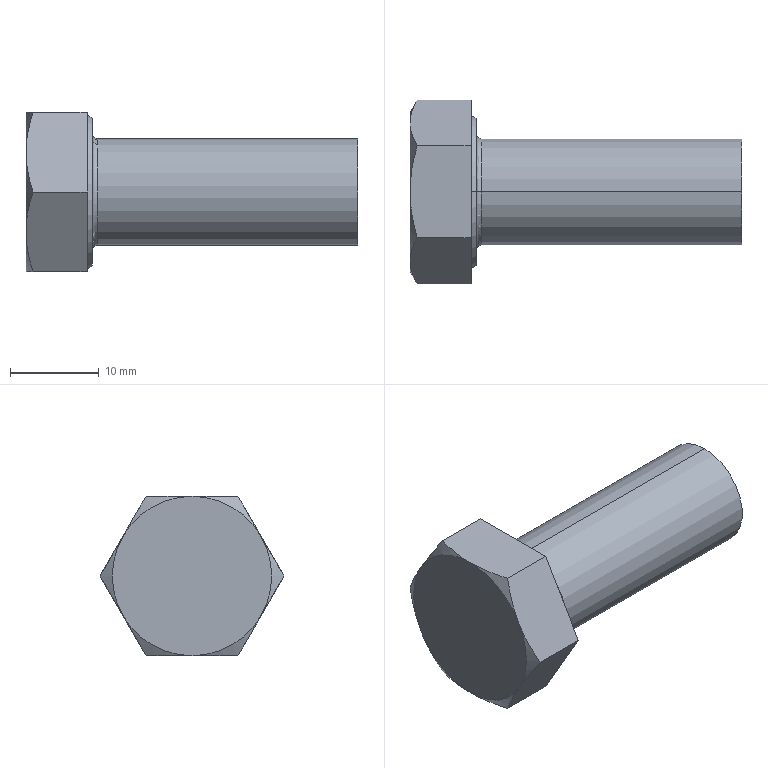Part | SolidWorks | features RevCut 3, Extrusion 1, Fillet 1, LPattern 1, Revolution 1 | 1 solid | 22 faces | box 37.5 x 20.785 x 18 mm | volume 5461 mm3 | plane 10 | cone 8 | torus 2 | cylinder 2 | commonest cylinder face diameters 12 x2
STEP:
#1=CARTESIAN_POINT('',(8.1,0.,6.));
#2=VERTEX_POINT('',#1);
#3=CARTESIAN_POINT('',(8.1,0.,-6.));
#4=VERTEX_POINT('',#3);
#5=CARTESIAN_POINT('',(8.1,0.,0.));
#6=DIRECTION('',(1.,0.,0.));
#7=DIRECTION('',(0.,0.,-1.));
#8=AXIS2_PLACEMENT_3D('',#5,#6,#7);
#9=CIRCLE('',#8,6.);
#10=EDGE_CURVE('',#2,#4,#9,.T.);
#11=ORIENTED_EDGE('',*,*,#10,.F.);
#12=CARTESIAN_POINT('',(7.5,0.,6.6));
#13=VERTEX_POINT('',#12);
#14=CARTESIAN_POINT('',(8.1,0.,6.6));
#15=DIRECTION('',(0.,1.,0.));
#16=DIRECTION('',(0.,0.,1.));
#17=AXIS2_PLACEMENT_3D('',#14,#15,#16);
#18=CIRCLE('',#17,0.6);
#19=EDGE_CURVE('',#2,#13,#18,.T.);
#20=ORIENTED_EDGE('',*,*,#19,.T.);
#21=CARTESIAN_POINT('',(7.5,0.,-6.6));
#22=VERTEX_POINT('',#21);
#23=CARTESIAN_POINT('',(7.5,0.,0.));
#24=DIRECTION('',(-1.,0.,0.));
#25=DIRECTION('',(0.,0.,-1.));
#26=AXIS2_PLACEMENT_3D('',#23,#24,#25);
#27=CIRCLE('',#26,6.6);
#28=EDGE_CURVE('',#22,#13,#27,.T.);
#29=ORIENTED_EDGE('',*,*,#28,.F.);
#30=CARTESIAN_POINT('',(8.1,0.,-6.6));
#31=DIRECTION('',(0.,-1.,0.));
#32=DIRECTION('',(0.,0.,-1.));
#33=AXIS2_PLACEMENT_3D('',#30,#31,#32);
#34=CIRCLE('',#33,0.6);
#35=EDGE_CURVE('',#4,#22,#34,.T.);
#36=ORIENTED_EDGE('',*,*,#35,.F.);
#37=EDGE_LOOP('',(#11,#20,#29,#36));
#38=FACE_OUTER_BOUND('',#37,.T.);
#39=CARTESIAN_POINT('',(8.1,0.,0.));
#40=DIRECTION('',(1.,0.,0.));
#41=DIRECTION('',(0.,0.,-1.));
#42=AXIS2_PLACEMENT_3D('',#39,#40,#41);
#43=TOROIDAL_SURFACE('',#42,6.6,0.6);
#44=ADVANCED_FACE('',(#38),#43,.F.);
#45=CARTESIAN_POINT('',(37.5,0.,6.));
#46=VERTEX_POINT('',#45);
#47=CARTESIAN_POINT('',(37.5,0.,-6.));
#48=VERTEX_POINT('',#47);
#49=CARTESIAN_POINT('',(37.5,0.,0.));
#50=DIRECTION('',(-1.,0.,0.));
#51=DIRECTION('',(0.,0.,1.));
#52=AXIS2_PLACEMENT_3D('',#49,#50,#51);
#53=CIRCLE('',#52,6.);
#54=EDGE_CURVE('',#46,#48,#53,.T.);
#55=ORIENTED_EDGE('',*,*,#54,.T.);
#56=CARTESIAN_POINT('',(0.,0.,-6.));
#57=DIRECTION('',(-1.,0.,0.));
#58=VECTOR('',#57,1000.);
#59=LINE('',#56,#58);
#60=EDGE_CURVE('',#48,#4,#59,.T.);
#61=ORIENTED_EDGE('',*,*,#60,.T.);
#62=CARTESIAN_POINT('',(8.1,0.,0.));
#63=DIRECTION('',(1.,0.,0.));
#64=DIRECTION('',(0.,0.,-1.));
#65=AXIS2_PLACEMENT_3D('',#62,#63,#64);
#66=CIRCLE('',#65,6.);
#67=EDGE_CURVE('',#4,#2,#66,.T.);
#68=ORIENTED_EDGE('',*,*,#67,.T.);
#69=CARTESIAN_POINT('',(0.,0.,6.));
#70=DIRECTION('',(-1.,0.,0.));
#71=VECTOR('',#70,1000.);
#72=LINE('',#69,#71);
#73=EDGE_CURVE('',#46,#2,#72,.T.);
#74=ORIENTED_EDGE('',*,*,#73,.F.);
#75=EDGE_LOOP('',(#55,#61,#68,#74));
#76=FACE_OUTER_BOUND('',#75,.T.);
#77=CARTESIAN_POINT('',(0.,0.,0.));
#78=DIRECTION('',(-1.,0.,0.));
#79=DIRECTION('',(0.,0.,1.));
#80=AXIS2_PLACEMENT_3D('',#77,#78,#79);
#81=CYLINDRICAL_SURFACE('',#80,6.);
#82=ADVANCED_FACE('',(#76),#81,.T.);
#83=CARTESIAN_POINT('',(7.5,0.,8.315));
#84=VERTEX_POINT('',#83);
#85=CARTESIAN_POINT('',(7.5,0.,-8.315));
#86=VERTEX_POINT('',#85);
#87=CARTESIAN_POINT('',(7.5,0.,0.));
#88=DIRECTION('',(-1.,0.,0.));
#89=DIRECTION('',(0.,0.,1.));
#90=AXIS2_PLACEMENT_3D('',#87,#88,#89);
#91=CIRCLE('',#90,8.315);
#92=EDGE_CURVE('',#84,#86,#91,.T.);
#93=ORIENTED_EDGE('',*,*,#92,.T.);
#94=CARTESIAN_POINT('',(6.9,0.,-8.661));
#95=VERTEX_POINT('',#94);
#96=CARTESIAN_POINT('',(6.9,0.,-8.661));
#97=DIRECTION('',(-0.866,0.,-0.5));
#98=VECTOR('',#97,1000.);
#99=LINE('',#96,#98);
#100=EDGE_CURVE('',#86,#95,#99,.T.);
#101=ORIENTED_EDGE('',*,*,#100,.T.);
#102=CARTESIAN_POINT('',(6.9,0.,8.661));
#103=VERTEX_POINT('',#102);
#104=CARTESIAN_POINT('',(6.9,0.,0.));
#105=DIRECTION('',(-1.,0.,0.));
#106=DIRECTION('',(0.,0.,1.));
#107=AXIS2_PLACEMENT_3D('',#104,#105,#106);
#108=CIRCLE('',#107,8.661);
#109=EDGE_CURVE('',#103,#95,#108,.T.);
#110=ORIENTED_EDGE('',*,*,#109,.F.);
#111=CARTESIAN_POINT('',(6.9,0.,8.661));
#112=DIRECTION('',(-0.866,0.,0.5));
#113=VECTOR('',#112,1000.);
#114=LINE('',#111,#113);
#115=EDGE_CURVE('',#84,#103,#114,.T.);
#116=ORIENTED_EDGE('',*,*,#115,.F.);
#117=EDGE_LOOP('',(#93,#101,#110,#116));
#118=FACE_OUTER_BOUND('',#117,.T.);
#119=CARTESIAN_POINT('',(6.9,0.,0.));
#120=DIRECTION('',(-1.,0.,0.));
#121=DIRECTION('',(0.,0.,1.));
#122=AXIS2_PLACEMENT_3D('',#119,#120,#121);
#123=CONICAL_SURFACE('',#122,8.661,0.5236);
#124=ADVANCED_FACE('',(#118),#123,.T.);
#125=CARTESIAN_POINT('',(6.9,5.196,-9.));
#126=VERTEX_POINT('',#125);
#127=CARTESIAN_POINT('',(6.9,10.392,0.));
#128=VERTEX_POINT('',#127);
#129=CARTESIAN_POINT('',(6.9,5.196,-9.));
#130=DIRECTION('',(0.,0.5,0.866));
#131=VECTOR('',#130,1000.);
#132=LINE('',#129,#131);
#133=EDGE_CURVE('',#126,#128,#132,.T.);
#134=ORIENTED_EDGE('',*,*,#133,.F.);
#135=CARTESIAN_POINT('',(0.8038,5.196,-9.));
#136=VERTEX_POINT('',#135);
#137=CARTESIAN_POINT('',(7.5,5.196,-9.));
#138=DIRECTION('',(-1.,0.,0.));
#139=VECTOR('',#138,1000.);
#140=LINE('',#137,#139);
#141=EDGE_CURVE('',#126,#136,#140,.T.);
#142=ORIENTED_EDGE('',*,*,#141,.T.);
#143=CARTESIAN_POINT('',(0.,7.794,-4.5));
#144=VERTEX_POINT('',#143);
#145=CARTESIAN_POINT('',(0.,7.794,-4.5));
#146=CARTESIAN_POINT('',(0.,7.574,-4.882));
#147=CARTESIAN_POINT('',(0.019,7.352,-5.266));
#148=CARTESIAN_POINT('',(0.09253,6.914,-6.024));
#149=CARTESIAN_POINT('',(0.147,6.697,-6.401));
#150=CARTESIAN_POINT('',(0.357,6.048,-7.525));
#151=CARTESIAN_POINT('',(0.5591,5.62,-8.266));
#152=CARTESIAN_POINT('',(0.8038,5.196,-9.));
#153=B_SPLINE_CURVE_WITH_KNOTS('',3,(#145,#146,#147,#148,#149,#150,#151,#152),.UNSPECIFIED.,.F.,.F.,(4,2,2,4),(0.005258,0.006567,0.007877,0.0105),.UNSPECIFIED.);
#154=EDGE_CURVE('',#144,#136,#153,.T.);
#155=ORIENTED_EDGE('',*,*,#154,.F.);
#156=CARTESIAN_POINT('',(0.8038,10.392,0.));
#157=VERTEX_POINT('',#156);
#158=CARTESIAN_POINT('',(0.8038,10.392,0.));
#159=CARTESIAN_POINT('',(0.5585,9.967,-0.7361));
#160=CARTESIAN_POINT('',(0.3563,9.539,-1.478));
#161=CARTESIAN_POINT('',(0.07661,8.674,-2.976));
#162=CARTESIAN_POINT('',(0.,8.237,-3.733));
#163=CARTESIAN_POINT('',(0.,7.794,-4.5));
#164=B_SPLINE_CURVE_WITH_KNOTS('',3,(#158,#159,#160,#161,#162,#163),.UNSPECIFIED.,.F.,.F.,(4,2,4),(0.000000238,0.002629,0.005258),.UNSPECIFIED.);
#165=EDGE_CURVE('',#157,#144,#164,.T.);
#166=ORIENTED_EDGE('',*,*,#165,.F.);
#167=CARTESIAN_POINT('',(7.5,10.392,0.));
#168=DIRECTION('',(-1.,0.,0.));
#169=VECTOR('',#168,1000.);
#170=LINE('',#167,#169);
#171=EDGE_CURVE('',#128,#157,#170,.T.);
#172=ORIENTED_EDGE('',*,*,#171,.F.);
#173=EDGE_LOOP('',(#134,#142,#155,#166,#172));
#174=FACE_OUTER_BOUND('',#173,.T.);
#175=CARTESIAN_POINT('',(7.5,5.196,-9.));
#176=DIRECTION('',(0.,-0.866,0.5));
#177=DIRECTION('',(0.,-0.5,-0.866));
#178=AXIS2_PLACEMENT_3D('',#175,#176,#177);
#179=PLANE('',#178);
#180=ADVANCED_FACE('',(#174),#179,.F.);
#181=CARTESIAN_POINT('',(6.9,5.196,9.));
#182=VERTEX_POINT('',#181);
#183=CARTESIAN_POINT('',(6.9,10.392,0.));
#184=DIRECTION('',(0.,-0.5,0.866));
#185=VECTOR('',#184,1000.);
#186=LINE('',#183,#185);
#187=EDGE_CURVE('',#128,#182,#186,.T.);
#188=ORIENTED_EDGE('',*,*,#187,.F.);
#189=ORIENTED_EDGE('',*,*,#171,.T.);
#190=CARTESIAN_POINT('',(0.,7.794,4.5));
#191=VERTEX_POINT('',#190);
#192=CARTESIAN_POINT('',(0.,7.794,4.5));
#193=CARTESIAN_POINT('',(0.,8.015,4.118));
#194=CARTESIAN_POINT('',(0.019,8.236,3.734));
#195=CARTESIAN_POINT('',(0.09253,8.674,2.976));
#196=CARTESIAN_POINT('',(0.147,8.892,2.599));
#197=CARTESIAN_POINT('',(0.357,9.541,1.475));
#198=CARTESIAN_POINT('',(0.5591,9.968,0.7343));
#199=CARTESIAN_POINT('',(0.8038,10.392,0.));
#200=B_SPLINE_CURVE_WITH_KNOTS('',3,(#192,#193,#194,#195,#196,#197,#198,#199),.UNSPECIFIED.,.F.,.F.,(4,2,2,4),(0.005258,0.006567,0.007877,0.0105),.UNSPECIFIED.);
#201=EDGE_CURVE('',#191,#157,#200,.T.);
#202=ORIENTED_EDGE('',*,*,#201,.F.);
#203=CARTESIAN_POINT('',(0.8038,5.196,9.));
#204=VERTEX_POINT('',#203);
#205=CARTESIAN_POINT('',(0.8038,5.196,9.));
#206=CARTESIAN_POINT('',(0.5585,5.621,8.264));
#207=CARTESIAN_POINT('',(0.3563,6.049,7.522));
#208=CARTESIAN_POINT('',(0.07661,6.914,6.024));
#209=CARTESIAN_POINT('',(0.,7.352,5.267));
#210=CARTESIAN_POINT('',(0.,7.794,4.5));
#211=B_SPLINE_CURVE_WITH_KNOTS('',3,(#205,#206,#207,#208,#209,#210),.UNSPECIFIED.,.F.,.F.,(4,2,4),(0.000000238,0.002629,0.005258),.UNSPECIFIED.);
#212=EDGE_CURVE('',#204,#191,#211,.T.);
#213=ORIENTED_EDGE('',*,*,#212,.F.);
#214=CARTESIAN_POINT('',(7.5,5.196,9.));
#215=DIRECTION('',(-1.,0.,0.));
#216=VECTOR('',#215,1000.);
#217=LINE('',#214,#216);
#218=EDGE_CURVE('',#182,#204,#217,.T.);
#219=ORIENTED_EDGE('',*,*,#218,.F.);
#220=EDGE_LOOP('',(#188,#189,#202,#213,#219));
#221=FACE_OUTER_BOUND('',#220,.T.);
#222=CARTESIAN_POINT('',(7.5,10.392,0.));
#223=DIRECTION('',(0.,-0.866,-0.5));
#224=DIRECTION('',(0.,0.5,-0.866));
#225=AXIS2_PLACEMENT_3D('',#222,#223,#224);
#226=PLANE('',#225);
#227=ADVANCED_FACE('',(#221),#226,.F.);
#228=CARTESIAN_POINT('',(6.9,-5.196,9.));
#229=VERTEX_POINT('',#228);
#230=CARTESIAN_POINT('',(6.9,5.196,9.));
#231=DIRECTION('',(0.,-1.,0.));
#232=VECTOR('',#231,1000.);
#233=LINE('',#230,#232);
#234=EDGE_CURVE('',#182,#229,#233,.T.);
#235=ORIENTED_EDGE('',*,*,#234,.F.);
#236=ORIENTED_EDGE('',*,*,#218,.T.);
#237=CARTESIAN_POINT('',(0.,0.,9.));
#238=VERTEX_POINT('',#237);
#239=CARTESIAN_POINT('',(0.,0.,9.));
#240=CARTESIAN_POINT('',(0.,0.4401,9.));
#241=CARTESIAN_POINT('',(0.01885,0.8832,9.));
#242=CARTESIAN_POINT('',(0.09319,1.767,9.));
#243=CARTESIAN_POINT('',(0.1482,2.204,9.));
#244=CARTESIAN_POINT('',(0.3593,3.505,9.));
#245=CARTESIAN_POINT('',(0.5612,4.356,9.));
#246=CARTESIAN_POINT('',(0.8038,5.196,9.));
#247=B_SPLINE_CURVE_WITH_KNOTS('',3,(#239,#240,#241,#242,#243,#244,#245,#246),.UNSPECIFIED.,.F.,.F.,(4,2,2,4),(0.01498,0.0163,0.01761,0.02025),.UNSPECIFIED.);
#248=EDGE_CURVE('',#238,#204,#247,.T.);
#249=ORIENTED_EDGE('',*,*,#248,.F.);
#250=CARTESIAN_POINT('',(0.8038,-5.196,9.));
#251=VERTEX_POINT('',#250);
#252=CARTESIAN_POINT('',(0.8038,-5.196,9.));
#253=CARTESIAN_POINT('',(0.5595,-4.35,9.));
#254=CARTESIAN_POINT('',(0.3552,-3.485,9.));
#255=CARTESIAN_POINT('',(0.07569,-1.752,9.));
#256=CARTESIAN_POINT('',(0.,-0.8794,9.));
#257=CARTESIAN_POINT('',(0.,0.,9.));
#258=B_SPLINE_CURVE_WITH_KNOTS('',3,(#252,#253,#254,#255,#256,#257),.UNSPECIFIED.,.F.,.F.,(4,2,4),(0.00972,0.01235,0.01498),.UNSPECIFIED.);
#259=EDGE_CURVE('',#251,#238,#258,.T.);
#260=ORIENTED_EDGE('',*,*,#259,.F.);
#261=CARTESIAN_POINT('',(7.5,-5.196,9.));
#262=DIRECTION('',(-1.,0.,0.));
#263=VECTOR('',#262,1000.);
#264=LINE('',#261,#263);
#265=EDGE_CURVE('',#229,#251,#264,.T.);
#266=ORIENTED_EDGE('',*,*,#265,.F.);
#267=EDGE_LOOP('',(#235,#236,#249,#260,#266));
#268=FACE_OUTER_BOUND('',#267,.T.);
#269=CARTESIAN_POINT('',(7.5,5.196,9.));
#270=DIRECTION('',(0.,0.,-1.));
#271=DIRECTION('',(-1.,0.,0.));
#272=AXIS2_PLACEMENT_3D('',#269,#270,#271);
#273=PLANE('',#272);
#274=ADVANCED_FACE('',(#268),#273,.F.);
#275=CARTESIAN_POINT('',(6.9,-10.392,0.));
#276=VERTEX_POINT('',#275);
#277=CARTESIAN_POINT('',(6.9,-10.392,0.));
#278=DIRECTION('',(0.,-0.5,-0.866));
#279=VECTOR('',#278,1000.);
#280=LINE('',#277,#279);
#281=EDGE_CURVE('',#229,#276,#280,.T.);
#282=ORIENTED_EDGE('',*,*,#281,.F.);
#283=ORIENTED_EDGE('',*,*,#265,.T.);
#284=CARTESIAN_POINT('',(0.,-7.794,4.5));
#285=VERTEX_POINT('',#284);
#286=CARTESIAN_POINT('',(0.,-7.794,4.5));
#287=CARTESIAN_POINT('',(0.,-7.574,4.882));
#288=CARTESIAN_POINT('',(0.019,-7.352,5.266));
#289=CARTESIAN_POINT('',(0.09253,-6.914,6.024));
#290=CARTESIAN_POINT('',(0.147,-6.697,6.401));
#291=CARTESIAN_POINT('',(0.357,-6.048,7.525));
#292=CARTESIAN_POINT('',(0.5591,-5.62,8.266));
#293=CARTESIAN_POINT('',(0.8038,-5.196,9.));
#294=B_SPLINE_CURVE_WITH_KNOTS('',3,(#286,#287,#288,#289,#290,#291,#292,#293),.UNSPECIFIED.,.F.,.F.,(4,2,2,4),(0.005258,0.006567,0.007877,0.0105),.UNSPECIFIED.);
#295=EDGE_CURVE('',#285,#251,#294,.T.);
#296=ORIENTED_EDGE('',*,*,#295,.F.);
#297=CARTESIAN_POINT('',(0.8038,-10.392,0.));
#298=VERTEX_POINT('',#297);
#299=CARTESIAN_POINT('',(0.8038,-10.392,0.));
#300=CARTESIAN_POINT('',(0.5585,-9.967,0.7361));
#301=CARTESIAN_POINT('',(0.3563,-9.539,1.478));
#302=CARTESIAN_POINT('',(0.07661,-8.674,2.976));
#303=CARTESIAN_POINT('',(0.,-8.237,3.733));
#304=CARTESIAN_POINT('',(0.,-7.794,4.5));
#305=B_SPLINE_CURVE_WITH_KNOTS('',3,(#299,#300,#301,#302,#303,#304),.UNSPECIFIED.,.F.,.F.,(4,2,4),(0.000000238,0.002629,0.005258),.UNSPECIFIED.);
#306=EDGE_CURVE('',#298,#285,#305,.T.);
#307=ORIENTED_EDGE('',*,*,#306,.F.);
#308=CARTESIAN_POINT('',(7.5,-10.392,0.));
#309=DIRECTION('',(-1.,0.,0.));
#310=VECTOR('',#309,1000.);
#311=LINE('',#308,#310);
#312=EDGE_CURVE('',#276,#298,#311,.T.);
#313=ORIENTED_EDGE('',*,*,#312,.F.);
#314=EDGE_LOOP('',(#282,#283,#296,#307,#313));
#315=FACE_OUTER_BOUND('',#314,.T.);
#316=CARTESIAN_POINT('',(7.5,-10.392,0.));
#317=DIRECTION('',(0.,0.866,-0.5));
#318=DIRECTION('',(0.,0.5,0.866));
#319=AXIS2_PLACEMENT_3D('',#316,#317,#318);
#320=PLANE('',#319);
#321=ADVANCED_FACE('',(#315),#320,.F.);
#322=CARTESIAN_POINT('',(6.9,-5.196,-9.));
#323=VERTEX_POINT('',#322);
#324=CARTESIAN_POINT('',(6.9,-5.196,-9.));
#325=DIRECTION('',(0.,0.5,-0.866));
#326=VECTOR('',#325,1000.);
#327=LINE('',#324,#326);
#328=EDGE_CURVE('',#276,#323,#327,.T.);
#329=ORIENTED_EDGE('',*,*,#328,.F.);
#330=ORIENTED_EDGE('',*,*,#312,.T.);
#331=CARTESIAN_POINT('',(0.,-7.794,-4.5));
#332=VERTEX_POINT('',#331);
#333=CARTESIAN_POINT('',(0.,-7.794,-4.5));
#334=CARTESIAN_POINT('',(0.,-8.015,-4.118));
#335=CARTESIAN_POINT('',(0.019,-8.236,-3.734));
#336=CARTESIAN_POINT('',(0.09253,-8.674,-2.976));
#337=CARTESIAN_POINT('',(0.147,-8.892,-2.599));
#338=CARTESIAN_POINT('',(0.357,-9.541,-1.475));
#339=CARTESIAN_POINT('',(0.5591,-9.968,-0.7343));
#340=CARTESIAN_POINT('',(0.8038,-10.392,0.));
#341=B_SPLINE_CURVE_WITH_KNOTS('',3,(#333,#334,#335,#336,#337,#338,#339,#340),.UNSPECIFIED.,.F.,.F.,(4,2,2,4),(0.005258,0.006567,0.007877,0.0105),.UNSPECIFIED.);
#342=EDGE_CURVE('',#332,#298,#341,.T.);
#343=ORIENTED_EDGE('',*,*,#342,.F.);
#344=CARTESIAN_POINT('',(0.8038,-5.196,-9.));
#345=VERTEX_POINT('',#344);
#346=CARTESIAN_POINT('',(0.8038,-5.196,-9.));
#347=CARTESIAN_POINT('',(0.5585,-5.621,-8.264));
#348=CARTESIAN_POINT('',(0.3563,-6.049,-7.522));
#349=CARTESIAN_POINT('',(0.07661,-6.914,-6.024));
#350=CARTESIAN_POINT('',(0.,-7.352,-5.267));
#351=CARTESIAN_POINT('',(0.,-7.794,-4.5));
#352=B_SPLINE_CURVE_WITH_KNOTS('',3,(#346,#347,#348,#349,#350,#351),.UNSPECIFIED.,.F.,.F.,(4,2,4),(0.000000238,0.002629,0.005258),.UNSPECIFIED.);
#353=EDGE_CURVE('',#345,#332,#352,.T.);
#354=ORIENTED_EDGE('',*,*,#353,.F.);
#355=CARTESIAN_POINT('',(7.5,-5.196,-9.));
#356=DIRECTION('',(-1.,0.,0.));
#357=VECTOR('',#356,1000.);
#358=LINE('',#355,#357);
#359=EDGE_CURVE('',#323,#345,#358,.T.);
#360=ORIENTED_EDGE('',*,*,#359,.F.);
#361=EDGE_LOOP('',(#329,#330,#343,#354,#360));
#362=FACE_OUTER_BOUND('',#361,.T.);
#363=CARTESIAN_POINT('',(7.5,-5.196,-9.));
#364=DIRECTION('',(0.,0.866,0.5));
#365=DIRECTION('',(0.,-0.5,0.866));
#366=AXIS2_PLACEMENT_3D('',#363,#364,#365);
#367=PLANE('',#366);
#368=ADVANCED_FACE('',(#362),#367,.F.);
#369=CARTESIAN_POINT('',(6.9,5.196,-9.));
#370=DIRECTION('',(0.,1.,0.));
#371=VECTOR('',#370,1000.);
#372=LINE('',#369,#371);
#373=EDGE_CURVE('',#323,#126,#372,.T.);
#374=ORIENTED_EDGE('',*,*,#373,.F.);
#375=ORIENTED_EDGE('',*,*,#359,.T.);
#376=CARTESIAN_POINT('',(0.,0.,-9.));
#377=VERTEX_POINT('',#376);
#378=CARTESIAN_POINT('',(0.,0.,-9.));
#379=CARTESIAN_POINT('',(0.,-0.8794,-9.));
#380=CARTESIAN_POINT('',(0.07569,-1.752,-9.));
#381=CARTESIAN_POINT('',(0.3552,-3.485,-9.));
#382=CARTESIAN_POINT('',(0.5595,-4.35,-9.));
#383=CARTESIAN_POINT('',(0.8038,-5.196,-9.));
#384=B_SPLINE_CURVE_WITH_KNOTS('',3,(#378,#379,#380,#381,#382,#383),.UNSPECIFIED.,.F.,.F.,(4,2,4),(0.03045,0.03308,0.03571),.UNSPECIFIED.);
#385=EDGE_CURVE('',#377,#345,#384,.T.);
#386=ORIENTED_EDGE('',*,*,#385,.F.);
#387=CARTESIAN_POINT('',(0.8038,5.196,-9.));
#388=CARTESIAN_POINT('',(0.5612,4.356,-9.));
#389=CARTESIAN_POINT('',(0.3593,3.505,-9.));
#390=CARTESIAN_POINT('',(0.1482,2.204,-9.));
#391=CARTESIAN_POINT('',(0.09319,1.767,-9.));
#392=CARTESIAN_POINT('',(0.01885,0.8832,-9.));
#393=CARTESIAN_POINT('',(0.,0.4401,-9.));
#394=CARTESIAN_POINT('',(0.,0.,-9.));
#395=B_SPLINE_CURVE_WITH_KNOTS('',3,(#387,#388,#389,#390,#391,#392,#393,#394),.UNSPECIFIED.,.F.,.F.,(4,2,2,4),(0.02519,0.02782,0.02914,0.03045),.UNSPECIFIED.);
#396=EDGE_CURVE('',#136,#377,#395,.T.);
#397=ORIENTED_EDGE('',*,*,#396,.F.);
#398=ORIENTED_EDGE('',*,*,#141,.F.);
#399=EDGE_LOOP('',(#374,#375,#386,#397,#398));
#400=FACE_OUTER_BOUND('',#399,.T.);
#401=CARTESIAN_POINT('',(7.5,5.196,-9.));
#402=DIRECTION('',(0.,0.,1.));
#403=DIRECTION('',(0.,-1.,0.));
#404=AXIS2_PLACEMENT_3D('',#401,#402,#403);
#405=PLANE('',#404);
#406=ADVANCED_FACE('',(#400),#405,.F.);
#407=ORIENTED_EDGE('',*,*,#353,.T.);
#408=CARTESIAN_POINT('',(0.,0.,0.));
#409=DIRECTION('',(1.,0.,0.));
#410=DIRECTION('',(0.,0.,-1.));
#411=AXIS2_PLACEMENT_3D('',#408,#409,#410);
#412=CIRCLE('',#411,9.);
#413=EDGE_CURVE('',#332,#377,#412,.T.);
#414=ORIENTED_EDGE('',*,*,#413,.T.);
#415=ORIENTED_EDGE('',*,*,#385,.T.);
#416=EDGE_LOOP('',(#407,#414,#415));
#417=FACE_OUTER_BOUND('',#416,.T.);
#418=CARTESIAN_POINT('',(0.,0.,0.));
#419=DIRECTION('',(1.,0.,0.));
#420=DIRECTION('',(0.,0.,-1.));
#421=AXIS2_PLACEMENT_3D('',#418,#419,#420);
#422=CONICAL_SURFACE('',#421,9.,1.047);
#423=ADVANCED_FACE('',(#417),#422,.T.);
#424=ORIENTED_EDGE('',*,*,#306,.T.);
#425=CARTESIAN_POINT('',(0.,0.,0.));
#426=DIRECTION('',(1.,0.,0.));
#427=DIRECTION('',(0.,0.,-1.));
#428=AXIS2_PLACEMENT_3D('',#425,#426,#427);
#429=CIRCLE('',#428,9.);
#430=EDGE_CURVE('',#285,#332,#429,.T.);
#431=ORIENTED_EDGE('',*,*,#430,.T.);
#432=ORIENTED_EDGE('',*,*,#342,.T.);
#433=EDGE_LOOP('',(#424,#431,#432));
#434=FACE_OUTER_BOUND('',#433,.T.);
#435=CARTESIAN_POINT('',(0.,0.,0.));
#436=DIRECTION('',(1.,0.,0.));
#437=DIRECTION('',(0.,0.,-1.));
#438=AXIS2_PLACEMENT_3D('',#435,#436,#437);
#439=CONICAL_SURFACE('',#438,9.,1.047);
#440=ADVANCED_FACE('',(#434),#439,.T.);
#441=ORIENTED_EDGE('',*,*,#259,.T.);
#442=CARTESIAN_POINT('',(0.,0.,0.));
#443=DIRECTION('',(1.,0.,0.));
#444=DIRECTION('',(0.,0.,-1.));
#445=AXIS2_PLACEMENT_3D('',#442,#443,#444);
#446=CIRCLE('',#445,9.);
#447=EDGE_CURVE('',#238,#285,#446,.T.);
#448=ORIENTED_EDGE('',*,*,#447,.T.);
#449=ORIENTED_EDGE('',*,*,#295,.T.);
#450=EDGE_LOOP('',(#441,#448,#449));
#451=FACE_OUTER_BOUND('',#450,.T.);
#452=CARTESIAN_POINT('',(0.,0.,0.));
#453=DIRECTION('',(1.,0.,0.));
#454=DIRECTION('',(0.,0.,-1.));
#455=AXIS2_PLACEMENT_3D('',#452,#453,#454);
#456=CONICAL_SURFACE('',#455,9.,1.047);
#457=ADVANCED_FACE('',(#451),#456,.T.);
#458=ORIENTED_EDGE('',*,*,#248,.T.);
#459=ORIENTED_EDGE('',*,*,#212,.T.);
#460=CARTESIAN_POINT('',(0.,0.,0.));
#461=DIRECTION('',(-1.,0.,0.));
#462=DIRECTION('',(0.,0.,1.));
#463=AXIS2_PLACEMENT_3D('',#460,#461,#462);
#464=CIRCLE('',#463,9.);
#465=EDGE_CURVE('',#238,#191,#464,.T.);
#466=ORIENTED_EDGE('',*,*,#465,.F.);
#467=EDGE_LOOP('',(#458,#459,#466));
#468=FACE_OUTER_BOUND('',#467,.T.);
#469=CARTESIAN_POINT('',(0.,0.,0.));
#470=DIRECTION('',(1.,0.,0.));
#471=DIRECTION('',(0.,0.,-1.));
#472=AXIS2_PLACEMENT_3D('',#469,#470,#471);
#473=CONICAL_SURFACE('',#472,9.,1.047);
#474=ADVANCED_FACE('',(#468),#473,.T.);
#475=ORIENTED_EDGE('',*,*,#201,.T.);
#476=ORIENTED_EDGE('',*,*,#165,.T.);
#477=CARTESIAN_POINT('',(0.,0.,0.));
#478=DIRECTION('',(1.,0.,0.));
#479=DIRECTION('',(0.,0.,-1.));
#480=AXIS2_PLACEMENT_3D('',#477,#478,#479);
#481=CIRCLE('',#480,9.);
#482=EDGE_CURVE('',#144,#191,#481,.T.);
#483=ORIENTED_EDGE('',*,*,#482,.T.);
#484=EDGE_LOOP('',(#475,#476,#483));
#485=FACE_OUTER_BOUND('',#484,.T.);
#486=CARTESIAN_POINT('',(0.,0.,0.));
#487=DIRECTION('',(1.,0.,0.));
#488=DIRECTION('',(0.,0.,-1.));
#489=AXIS2_PLACEMENT_3D('',#486,#487,#488);
#490=CONICAL_SURFACE('',#489,9.,1.047);
#491=ADVANCED_FACE('',(#485),#490,.T.);
#492=ORIENTED_EDGE('',*,*,#154,.T.);
#493=ORIENTED_EDGE('',*,*,#396,.T.);
#494=CARTESIAN_POINT('',(0.,0.,0.));
#495=DIRECTION('',(1.,0.,0.));
#496=DIRECTION('',(0.,0.,-1.));
#497=AXIS2_PLACEMENT_3D('',#494,#495,#496);
#498=CIRCLE('',#497,9.);
#499=EDGE_CURVE('',#377,#144,#498,.T.);
#500=ORIENTED_EDGE('',*,*,#499,.T.);
#501=EDGE_LOOP('',(#492,#493,#500));
#502=FACE_OUTER_BOUND('',#501,.T.);
#503=CARTESIAN_POINT('',(0.,0.,0.));
#504=DIRECTION('',(1.,0.,0.));
#505=DIRECTION('',(0.,0.,-1.));
#506=AXIS2_PLACEMENT_3D('',#503,#504,#505);
#507=CONICAL_SURFACE('',#506,9.,1.047);
#508=ADVANCED_FACE('',(#502),#507,.T.);
#509=ORIENTED_EDGE('',*,*,#499,.F.);
#510=ORIENTED_EDGE('',*,*,#413,.F.);
#511=ORIENTED_EDGE('',*,*,#430,.F.);
#512=ORIENTED_EDGE('',*,*,#447,.F.);
#513=ORIENTED_EDGE('',*,*,#465,.T.);
#514=ORIENTED_EDGE('',*,*,#482,.F.);
#515=EDGE_LOOP('',(#509,#510,#511,#512,#513,#514));
#516=FACE_OUTER_BOUND('',#515,.T.);
#517=CARTESIAN_POINT('',(0.,10.392,0.));
#518=DIRECTION('',(1.,0.,0.));
#519=DIRECTION('',(0.,0.,-1.));
#520=AXIS2_PLACEMENT_3D('',#517,#518,#519);
#521=PLANE('',#520);
#522=ADVANCED_FACE('',(#516),#521,.F.);
#523=ORIENTED_EDGE('',*,*,#109,.T.);
#524=CARTESIAN_POINT('',(6.9,0.,0.));
#525=DIRECTION('',(-1.,0.,0.));
#526=DIRECTION('',(0.,0.,1.));
#527=AXIS2_PLACEMENT_3D('',#524,#525,#526);
#528=CIRCLE('',#527,8.661);
#529=EDGE_CURVE('',#95,#103,#528,.T.);
#530=ORIENTED_EDGE('',*,*,#529,.T.);
#531=EDGE_LOOP('',(#523,#530));
#532=FACE_BOUND('',#531,.T.);
#533=ORIENTED_EDGE('',*,*,#133,.T.);
#534=ORIENTED_EDGE('',*,*,#187,.T.);
#535=ORIENTED_EDGE('',*,*,#234,.T.);
#536=ORIENTED_EDGE('',*,*,#281,.T.);
#537=ORIENTED_EDGE('',*,*,#328,.T.);
#538=ORIENTED_EDGE('',*,*,#373,.T.);
#539=EDGE_LOOP('',(#533,#534,#535,#536,#537,#538));
#540=FACE_OUTER_BOUND('',#539,.T.);
#541=CARTESIAN_POINT('',(6.9,8.661,0.));
#542=DIRECTION('',(1.,0.,0.));
#543=DIRECTION('',(0.,0.,-1.));
#544=AXIS2_PLACEMENT_3D('',#541,#542,#543);
#545=PLANE('',#544);
#546=ADVANCED_FACE('',(#532,#540),#545,.T.);
#547=ORIENTED_EDGE('',*,*,#100,.F.);
#548=CARTESIAN_POINT('',(7.5,0.,0.));
#549=DIRECTION('',(-1.,0.,0.));
#550=DIRECTION('',(0.,0.,1.));
#551=AXIS2_PLACEMENT_3D('',#548,#549,#550);
#552=CIRCLE('',#551,8.315);
#553=EDGE_CURVE('',#86,#84,#552,.T.);
#554=ORIENTED_EDGE('',*,*,#553,.T.);
#555=ORIENTED_EDGE('',*,*,#115,.T.);
#556=ORIENTED_EDGE('',*,*,#529,.F.);
#557=EDGE_LOOP('',(#547,#554,#555,#556));
#558=FACE_OUTER_BOUND('',#557,.T.);
#559=CARTESIAN_POINT('',(6.9,0.,0.));
#560=DIRECTION('',(-1.,0.,0.));
#561=DIRECTION('',(0.,0.,1.));
#562=AXIS2_PLACEMENT_3D('',#559,#560,#561);
#563=CONICAL_SURFACE('',#562,8.661,0.5236);
#564=ADVANCED_FACE('',(#558),#563,.T.);
#565=ORIENTED_EDGE('',*,*,#54,.F.);
#566=CARTESIAN_POINT('',(37.5,0.,0.));
#567=DIRECTION('',(-1.,0.,0.));
#568=DIRECTION('',(0.,0.,1.));
#569=AXIS2_PLACEMENT_3D('',#566,#567,#568);
#570=CIRCLE('',#569,6.);
#571=EDGE_CURVE('',#48,#46,#570,.T.);
#572=ORIENTED_EDGE('',*,*,#571,.F.);
#573=EDGE_LOOP('',(#565,#572));
#574=FACE_OUTER_BOUND('',#573,.T.);
#575=CARTESIAN_POINT('',(37.5,0.,0.));
#576=DIRECTION('',(-1.,0.,0.));
#577=DIRECTION('',(0.,0.,1.));
#578=AXIS2_PLACEMENT_3D('',#575,#576,#577);
#579=PLANE('',#578);
#580=ADVANCED_FACE('',(#574),#579,.F.);
#581=ORIENTED_EDGE('',*,*,#60,.F.);
#582=ORIENTED_EDGE('',*,*,#571,.T.);
#583=ORIENTED_EDGE('',*,*,#73,.T.);
#584=ORIENTED_EDGE('',*,*,#10,.T.);
#585=EDGE_LOOP('',(#581,#582,#583,#584));
#586=FACE_OUTER_BOUND('',#585,.T.);
#587=CARTESIAN_POINT('',(0.,0.,0.));
#588=DIRECTION('',(-1.,0.,0.));
#589=DIRECTION('',(0.,0.,1.));
#590=AXIS2_PLACEMENT_3D('',#587,#588,#589);
#591=CYLINDRICAL_SURFACE('',#590,6.);
#592=ADVANCED_FACE('',(#586),#591,.T.);
#593=ORIENTED_EDGE('',*,*,#28,.T.);
#594=CARTESIAN_POINT('',(7.5,0.,0.));
#595=DIRECTION('',(-1.,0.,0.));
#596=DIRECTION('',(0.,0.,-1.));
#597=AXIS2_PLACEMENT_3D('',#594,#595,#596);
#598=CIRCLE('',#597,6.6);
#599=EDGE_CURVE('',#13,#22,#598,.T.);
#600=ORIENTED_EDGE('',*,*,#599,.T.);
#601=EDGE_LOOP('',(#593,#600));
#602=FACE_BOUND('',#601,.T.);
#603=ORIENTED_EDGE('',*,*,#92,.F.);
#604=ORIENTED_EDGE('',*,*,#553,.F.);
#605=EDGE_LOOP('',(#603,#604));
#606=FACE_OUTER_BOUND('',#605,.T.);
#607=CARTESIAN_POINT('',(7.5,10.392,0.));
#608=DIRECTION('',(1.,0.,0.));
#609=DIRECTION('',(0.,0.,-1.));
#610=AXIS2_PLACEMENT_3D('',#607,#608,#609);
#611=PLANE('',#610);
#612=ADVANCED_FACE('',(#602,#606),#611,.T.);
#613=ORIENTED_EDGE('',*,*,#19,.F.);
#614=ORIENTED_EDGE('',*,*,#67,.F.);
#615=ORIENTED_EDGE('',*,*,#35,.T.);
#616=ORIENTED_EDGE('',*,*,#599,.F.);
#617=EDGE_LOOP('',(#613,#614,#615,#616));
#618=FACE_OUTER_BOUND('',#617,.T.);
#619=CARTESIAN_POINT('',(8.1,0.,0.));
#620=DIRECTION('',(1.,0.,0.));
#621=DIRECTION('',(0.,0.,-1.));
#622=AXIS2_PLACEMENT_3D('',#619,#620,#621);
#623=TOROIDAL_SURFACE('',#622,6.6,0.6);
#624=ADVANCED_FACE('',(#618),#623,.F.);
#625=CLOSED_SHELL('',(#44,#82,#124,#180,#227,#274,#321,#368,#406,#423,#440,#457,#474,#491,#508,#522,#546,#564,#580,#592,#612,#624));
#626=MANIFOLD_SOLID_BREP('',#625);
#627=CARTESIAN_POINT('',(0.,0.,0.));
#628=DIRECTION('',(0.,0.,1.));
#629=DIRECTION('',(1.,0.,0.));
#630=AXIS2_PLACEMENT_3D('',#627,#628,#629);
#631=(LENGTH_UNIT()NAMED_UNIT(*)SI_UNIT(.MILLI.,.METRE.));
#632=UNCERTAINTY_MEASURE_WITH_UNIT(LENGTH_MEASURE(0.00001),#631,'','');
#633=(NAMED_UNIT(*)PLANE_ANGLE_UNIT()SI_UNIT($,.RADIAN.));
#634=(NAMED_UNIT(*)SI_UNIT($,.STERADIAN.)SOLID_ANGLE_UNIT());
#635=(GEOMETRIC_REPRESENTATION_CONTEXT(3)GLOBAL_UNCERTAINTY_ASSIGNED_CONTEXT((#632))GLOBAL_UNIT_ASSIGNED_CONTEXT((#631,#633,#634))REPRESENTATION_CONTEXT('',''));
#636=ADVANCED_BREP_SHAPE_REPRESENTATION('',(#626,#630),#635);